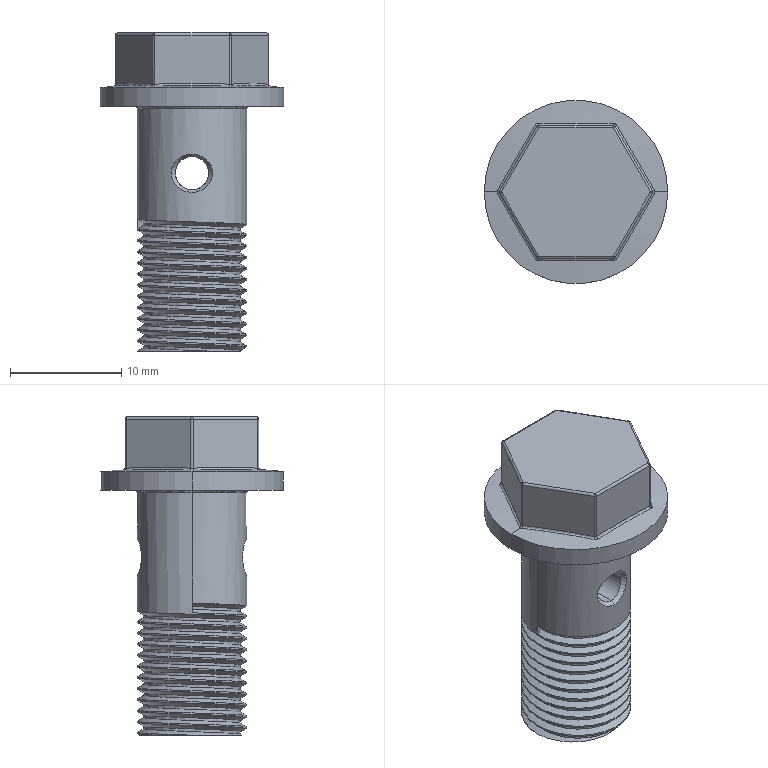Part | SolidWorks | features BaseBody 1 | 1 solid | 87 faces | box 16.5 x 16.5 x 28.623 mm | volume 2327 mm3 | cylinder 43 | spline 19 | plane 12 | sphere 7 | cone 4 | torus 2 | commonest cylinder face diameters 9.82 x24 0.4 x13 3 x2 3.4 x2 16.5 x2